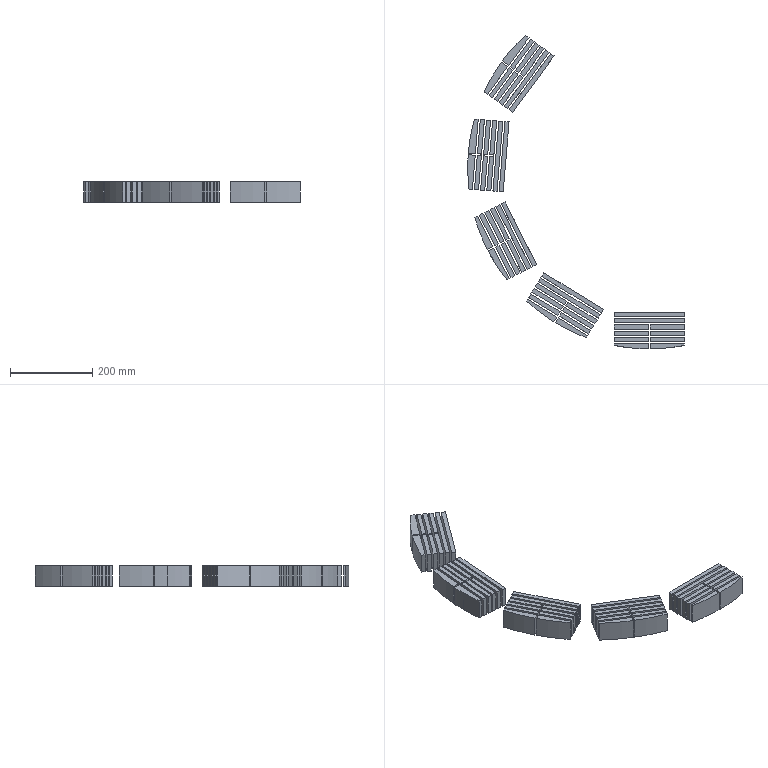Part | SolidWorks | features ICE 9, Extrusion 1 | 50 solids | 341 faces | box 525 x 761.019 x 50 mm | volume 2587889 mm3 | plane 290 | cylinder 51 | commonest cylinder face diameters 15 x40 880 x11